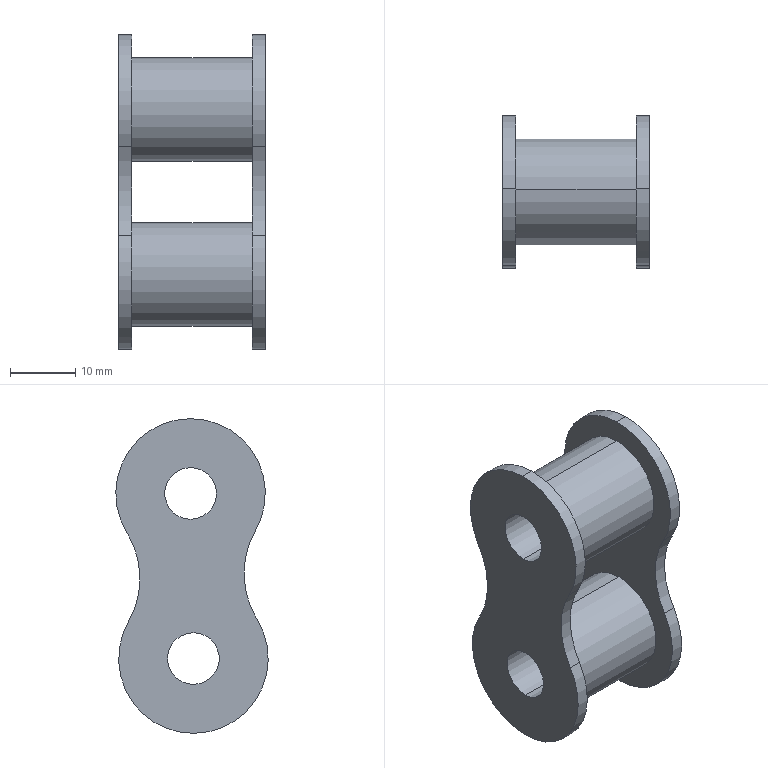Part | STEP file | Mirror 4 | 1 solid | 24 faces | box 22.5 x 23.441 x 48.396 mm | volume 8734 mm3 | cylinder 20 | plane 4 | commonest cylinder face diameters 23 x8 7.94 x4 15.88 x4 26.656 x4
STEP:
#1=CARTESIAN_POINT('',(346.684,-553.033,2506.288));
#2=VERTEX_POINT('',#1);
#3=CARTESIAN_POINT('',(346.684,-563.215,2489.079));
#4=VERTEX_POINT('',#3);
#5=CARTESIAN_POINT('',(346.684,-563.015,2500.578));
#6=DIRECTION('',(-1.,0.,0.));
#7=DIRECTION('',(0.,-0.01735,-0.9998));
#8=AXIS2_PLACEMENT_3D('',#5,#6,#7);
#9=CIRCLE('',#8,11.5);
#10=EDGE_CURVE('',#2,#4,#9,.T.);
#11=ORIENTED_EDGE('',*,*,#10,.T.);
#12=CARTESIAN_POINT('',(344.684,-563.215,2489.079));
#13=VERTEX_POINT('',#12);
#14=CARTESIAN_POINT('',(346.684,-563.215,2489.079));
#15=DIRECTION('',(-1.,0.,0.));
#16=VECTOR('',#15,1000.);
#17=LINE('',#14,#16);
#18=EDGE_CURVE('',#4,#13,#17,.T.);
#19=ORIENTED_EDGE('',*,*,#18,.T.);
#20=CARTESIAN_POINT('',(344.684,-553.033,2506.288));
#21=VERTEX_POINT('',#20);
#22=CARTESIAN_POINT('',(344.684,-563.015,2500.578));
#23=DIRECTION('',(-1.,0.,0.));
#24=DIRECTION('',(0.,-0.01735,-0.9998));
#25=AXIS2_PLACEMENT_3D('',#22,#23,#24);
#26=CIRCLE('',#25,11.5);
#27=EDGE_CURVE('',#21,#13,#26,.T.);
#28=ORIENTED_EDGE('',*,*,#27,.F.);
#29=CARTESIAN_POINT('',(346.684,-553.033,2506.288));
#30=DIRECTION('',(-1.,0.,0.));
#31=VECTOR('',#30,1000.);
#32=LINE('',#29,#31);
#33=EDGE_CURVE('',#2,#21,#32,.T.);
#34=ORIENTED_EDGE('',*,*,#33,.F.);
#35=EDGE_LOOP('',(#11,#19,#28,#34));
#36=FACE_OUTER_BOUND('',#35,.T.);
#37=CARTESIAN_POINT('',(346.684,-563.015,2500.578));
#38=DIRECTION('',(-1.,0.,0.));
#39=DIRECTION('',(0.,-0.01735,-0.9998));
#40=AXIS2_PLACEMENT_3D('',#37,#38,#39);
#41=CYLINDRICAL_SURFACE('',#40,11.5);
#42=ADVANCED_FACE('',(#36),#41,.T.);
#43=CARTESIAN_POINT('',(365.184,-563.215,2489.079));
#44=VERTEX_POINT('',#43);
#45=CARTESIAN_POINT('',(365.184,-572.793,2506.631));
#46=VERTEX_POINT('',#45);
#47=CARTESIAN_POINT('',(365.184,-563.015,2500.578));
#48=DIRECTION('',(-1.,0.,0.));
#49=DIRECTION('',(0.,-0.01735,-0.9998));
#50=AXIS2_PLACEMENT_3D('',#47,#48,#49);
#51=CIRCLE('',#50,11.5);
#52=EDGE_CURVE('',#44,#46,#51,.T.);
#53=ORIENTED_EDGE('',*,*,#52,.F.);
#54=CARTESIAN_POINT('',(367.184,-563.215,2489.079));
#55=VERTEX_POINT('',#54);
#56=CARTESIAN_POINT('',(365.184,-563.215,2489.079));
#57=DIRECTION('',(1.,0.,0.));
#58=VECTOR('',#57,1000.);
#59=LINE('',#56,#58);
#60=EDGE_CURVE('',#44,#55,#59,.T.);
#61=ORIENTED_EDGE('',*,*,#60,.T.);
#62=CARTESIAN_POINT('',(367.184,-572.793,2506.631));
#63=VERTEX_POINT('',#62);
#64=CARTESIAN_POINT('',(367.184,-563.015,2500.578));
#65=DIRECTION('',(-1.,0.,0.));
#66=DIRECTION('',(0.,-0.01735,-0.9998));
#67=AXIS2_PLACEMENT_3D('',#64,#65,#66);
#68=CIRCLE('',#67,11.5);
#69=EDGE_CURVE('',#55,#63,#68,.T.);
#70=ORIENTED_EDGE('',*,*,#69,.T.);
#71=CARTESIAN_POINT('',(365.184,-572.793,2506.631));
#72=DIRECTION('',(1.,0.,0.));
#73=VECTOR('',#72,1000.);
#74=LINE('',#71,#73);
#75=EDGE_CURVE('',#46,#63,#74,.T.);
#76=ORIENTED_EDGE('',*,*,#75,.F.);
#77=EDGE_LOOP('',(#53,#61,#70,#76));
#78=FACE_OUTER_BOUND('',#77,.T.);
#79=CARTESIAN_POINT('',(365.184,-563.015,2500.578));
#80=DIRECTION('',(1.,0.,0.));
#81=DIRECTION('',(0.,-0.01735,-0.9998));
#82=AXIS2_PLACEMENT_3D('',#79,#80,#81);
#83=CYLINDRICAL_SURFACE('',#82,11.5);
#84=ADVANCED_FACE('',(#78),#83,.T.);
#85=CARTESIAN_POINT('',(346.684,-572.557,2520.264));
#86=VERTEX_POINT('',#85);
#87=CARTESIAN_POINT('',(346.684,-562.375,2537.472));
#88=VERTEX_POINT('',#87);
#89=CARTESIAN_POINT('',(346.684,-562.574,2525.974));
#90=DIRECTION('',(-1.,0.,0.));
#91=DIRECTION('',(0.,-0.01735,-0.9998));
#92=AXIS2_PLACEMENT_3D('',#89,#90,#91);
#93=CIRCLE('',#92,11.5);
#94=EDGE_CURVE('',#86,#88,#93,.T.);
#95=ORIENTED_EDGE('',*,*,#94,.T.);
#96=CARTESIAN_POINT('',(344.684,-562.375,2537.472));
#97=VERTEX_POINT('',#96);
#98=CARTESIAN_POINT('',(346.684,-562.375,2537.472));
#99=DIRECTION('',(-1.,0.,0.));
#100=VECTOR('',#99,1000.);
#101=LINE('',#98,#100);
#102=EDGE_CURVE('',#88,#97,#101,.T.);
#103=ORIENTED_EDGE('',*,*,#102,.T.);
#104=CARTESIAN_POINT('',(344.684,-572.557,2520.264));
#105=VERTEX_POINT('',#104);
#106=CARTESIAN_POINT('',(344.684,-562.574,2525.974));
#107=DIRECTION('',(-1.,0.,0.));
#108=DIRECTION('',(0.,-0.01735,-0.9998));
#109=AXIS2_PLACEMENT_3D('',#106,#107,#108);
#110=CIRCLE('',#109,11.5);
#111=EDGE_CURVE('',#105,#97,#110,.T.);
#112=ORIENTED_EDGE('',*,*,#111,.F.);
#113=CARTESIAN_POINT('',(346.684,-572.557,2520.264));
#114=DIRECTION('',(-1.,0.,0.));
#115=VECTOR('',#114,1000.);
#116=LINE('',#113,#115);
#117=EDGE_CURVE('',#86,#105,#116,.T.);
#118=ORIENTED_EDGE('',*,*,#117,.F.);
#119=EDGE_LOOP('',(#95,#103,#112,#118));
#120=FACE_OUTER_BOUND('',#119,.T.);
#121=CARTESIAN_POINT('',(346.684,-562.574,2525.974));
#122=DIRECTION('',(-1.,0.,0.));
#123=DIRECTION('',(0.,-0.01735,-0.9998));
#124=AXIS2_PLACEMENT_3D('',#121,#122,#123);
#125=CYLINDRICAL_SURFACE('',#124,11.5);
#126=ADVANCED_FACE('',(#120),#125,.T.);
#127=CARTESIAN_POINT('',(346.684,-563.153,2492.639));
#128=VERTEX_POINT('',#127);
#129=CARTESIAN_POINT('',(346.684,-562.877,2508.516));
#130=VERTEX_POINT('',#129);
#131=CARTESIAN_POINT('',(346.684,-563.015,2500.578));
#132=DIRECTION('',(-1.,0.,0.));
#133=DIRECTION('',(0.,0.01735,0.9998));
#134=AXIS2_PLACEMENT_3D('',#131,#132,#133);
#135=CIRCLE('',#134,7.94);
#136=EDGE_CURVE('',#128,#130,#135,.T.);
#137=ORIENTED_EDGE('',*,*,#136,.F.);
#138=CARTESIAN_POINT('',(365.184,-563.153,2492.639));
#139=VERTEX_POINT('',#138);
#140=CARTESIAN_POINT('',(355.934,-563.153,2492.639));
#141=DIRECTION('',(-1.,0.,0.));
#142=VECTOR('',#141,1000.);
#143=LINE('',#140,#142);
#144=EDGE_CURVE('',#139,#128,#143,.T.);
#145=ORIENTED_EDGE('',*,*,#144,.F.);
#146=CARTESIAN_POINT('',(365.184,-562.877,2508.516));
#147=VERTEX_POINT('',#146);
#148=CARTESIAN_POINT('',(365.184,-563.015,2500.578));
#149=DIRECTION('',(-1.,0.,0.));
#150=DIRECTION('',(0.,0.01735,0.9998));
#151=AXIS2_PLACEMENT_3D('',#148,#149,#150);
#152=CIRCLE('',#151,7.94);
#153=EDGE_CURVE('',#139,#147,#152,.T.);
#154=ORIENTED_EDGE('',*,*,#153,.T.);
#155=CARTESIAN_POINT('',(355.934,-562.877,2508.516));
#156=DIRECTION('',(-1.,0.,0.));
#157=VECTOR('',#156,1000.);
#158=LINE('',#155,#157);
#159=EDGE_CURVE('',#147,#130,#158,.T.);
#160=ORIENTED_EDGE('',*,*,#159,.T.);
#161=EDGE_LOOP('',(#137,#145,#154,#160));
#162=FACE_OUTER_BOUND('',#161,.T.);
#163=CARTESIAN_POINT('',(355.934,-563.015,2500.578));
#164=DIRECTION('',(1.,0.,0.));
#165=DIRECTION('',(0.,-0.01735,-0.9998));
#166=AXIS2_PLACEMENT_3D('',#163,#164,#165);
#167=CYLINDRICAL_SURFACE('',#166,7.94);
#168=ADVANCED_FACE('',(#162),#167,.T.);
#169=CARTESIAN_POINT('',(346.684,-562.712,2518.035));
#170=VERTEX_POINT('',#169);
#171=CARTESIAN_POINT('',(346.684,-562.437,2533.913));
#172=VERTEX_POINT('',#171);
#173=CARTESIAN_POINT('',(346.684,-562.574,2525.974));
#174=DIRECTION('',(-1.,0.,0.));
#175=DIRECTION('',(0.,-0.01735,-0.9998));
#176=AXIS2_PLACEMENT_3D('',#173,#174,#175);
#177=CIRCLE('',#176,7.94);
#178=EDGE_CURVE('',#170,#172,#177,.T.);
#179=ORIENTED_EDGE('',*,*,#178,.F.);
#180=CARTESIAN_POINT('',(365.184,-562.712,2518.035));
#181=VERTEX_POINT('',#180);
#182=CARTESIAN_POINT('',(355.934,-562.712,2518.035));
#183=DIRECTION('',(-1.,0.,0.));
#184=VECTOR('',#183,1000.);
#185=LINE('',#182,#184);
#186=EDGE_CURVE('',#181,#170,#185,.T.);
#187=ORIENTED_EDGE('',*,*,#186,.F.);
#188=CARTESIAN_POINT('',(365.184,-562.437,2533.913));
#189=VERTEX_POINT('',#188);
#190=CARTESIAN_POINT('',(365.184,-562.574,2525.974));
#191=DIRECTION('',(-1.,0.,0.));
#192=DIRECTION('',(0.,-0.01735,-0.9998));
#193=AXIS2_PLACEMENT_3D('',#190,#191,#192);
#194=CIRCLE('',#193,7.94);
#195=EDGE_CURVE('',#181,#189,#194,.T.);
#196=ORIENTED_EDGE('',*,*,#195,.T.);
#197=CARTESIAN_POINT('',(355.934,-562.437,2533.913));
#198=DIRECTION('',(-1.,0.,0.));
#199=VECTOR('',#198,1000.);
#200=LINE('',#197,#199);
#201=EDGE_CURVE('',#189,#172,#200,.T.);
#202=ORIENTED_EDGE('',*,*,#201,.T.);
#203=EDGE_LOOP('',(#179,#187,#196,#202));
#204=FACE_OUTER_BOUND('',#203,.T.);
#205=CARTESIAN_POINT('',(355.934,-562.574,2525.974));
#206=DIRECTION('',(1.,0.,0.));
#207=DIRECTION('',(0.,-0.01735,-0.9998));
#208=AXIS2_PLACEMENT_3D('',#205,#206,#207);
#209=CYLINDRICAL_SURFACE('',#208,7.94);
#210=ADVANCED_FACE('',(#204),#209,.T.);
#211=CARTESIAN_POINT('',(367.184,-562.506,2529.943));
#212=VERTEX_POINT('',#211);
#213=CARTESIAN_POINT('',(367.184,-562.643,2522.004));
#214=VERTEX_POINT('',#213);
#215=CARTESIAN_POINT('',(367.184,-562.574,2525.974));
#216=DIRECTION('',(-1.,0.,0.));
#217=DIRECTION('',(0.,-0.01735,-0.9998));
#218=AXIS2_PLACEMENT_3D('',#215,#216,#217);
#219=CIRCLE('',#218,3.97);
#220=EDGE_CURVE('',#212,#214,#219,.T.);
#221=ORIENTED_EDGE('',*,*,#220,.F.);
#222=CARTESIAN_POINT('',(344.684,-562.506,2529.943));
#223=VERTEX_POINT('',#222);
#224=CARTESIAN_POINT('',(367.184,-562.506,2529.943));
#225=DIRECTION('',(-1.,0.,0.));
#226=VECTOR('',#225,1000.);
#227=LINE('',#224,#226);
#228=EDGE_CURVE('',#212,#223,#227,.T.);
#229=ORIENTED_EDGE('',*,*,#228,.T.);
#230=CARTESIAN_POINT('',(344.684,-562.643,2522.004));
#231=VERTEX_POINT('',#230);
#232=CARTESIAN_POINT('',(344.684,-562.574,2525.974));
#233=DIRECTION('',(-1.,0.,0.));
#234=DIRECTION('',(0.,-0.01735,-0.9998));
#235=AXIS2_PLACEMENT_3D('',#232,#233,#234);
#236=CIRCLE('',#235,3.97);
#237=EDGE_CURVE('',#223,#231,#236,.T.);
#238=ORIENTED_EDGE('',*,*,#237,.T.);
#239=CARTESIAN_POINT('',(367.184,-562.643,2522.004));
#240=DIRECTION('',(-1.,0.,0.));
#241=VECTOR('',#240,1000.);
#242=LINE('',#239,#241);
#243=EDGE_CURVE('',#214,#231,#242,.T.);
#244=ORIENTED_EDGE('',*,*,#243,.F.);
#245=EDGE_LOOP('',(#221,#229,#238,#244));
#246=FACE_OUTER_BOUND('',#245,.T.);
#247=CARTESIAN_POINT('',(367.184,-562.574,2525.974));
#248=DIRECTION('',(-1.,0.,0.));
#249=DIRECTION('',(0.,0.01735,0.9998));
#250=AXIS2_PLACEMENT_3D('',#247,#248,#249);
#251=CYLINDRICAL_SURFACE('',#250,3.97);
#252=ADVANCED_FACE('',(#246),#251,.F.);
#253=CARTESIAN_POINT('',(367.184,-562.946,2504.547));
#254=VERTEX_POINT('',#253);
#255=CARTESIAN_POINT('',(367.184,-563.084,2496.608));
#256=VERTEX_POINT('',#255);
#257=CARTESIAN_POINT('',(367.184,-563.015,2500.578));
#258=DIRECTION('',(-1.,0.,0.));
#259=DIRECTION('',(0.,0.01735,0.9998));
#260=AXIS2_PLACEMENT_3D('',#257,#258,#259);
#261=CIRCLE('',#260,3.97);
#262=EDGE_CURVE('',#254,#256,#261,.T.);
#263=ORIENTED_EDGE('',*,*,#262,.F.);
#264=CARTESIAN_POINT('',(344.684,-562.946,2504.547));
#265=VERTEX_POINT('',#264);
#266=CARTESIAN_POINT('',(367.184,-562.946,2504.547));
#267=DIRECTION('',(-1.,0.,0.));
#268=VECTOR('',#267,1000.);
#269=LINE('',#266,#268);
#270=EDGE_CURVE('',#254,#265,#269,.T.);
#271=ORIENTED_EDGE('',*,*,#270,.T.);
#272=CARTESIAN_POINT('',(344.684,-563.084,2496.608));
#273=VERTEX_POINT('',#272);
#274=CARTESIAN_POINT('',(344.684,-563.015,2500.578));
#275=DIRECTION('',(-1.,0.,0.));
#276=DIRECTION('',(0.,0.01735,0.9998));
#277=AXIS2_PLACEMENT_3D('',#274,#275,#276);
#278=CIRCLE('',#277,3.97);
#279=EDGE_CURVE('',#265,#273,#278,.T.);
#280=ORIENTED_EDGE('',*,*,#279,.T.);
#281=CARTESIAN_POINT('',(367.184,-563.084,2496.608));
#282=DIRECTION('',(-1.,0.,0.));
#283=VECTOR('',#282,1000.);
#284=LINE('',#281,#283);
#285=EDGE_CURVE('',#256,#273,#284,.T.);
#286=ORIENTED_EDGE('',*,*,#285,.F.);
#287=EDGE_LOOP('',(#263,#271,#280,#286));
#288=FACE_OUTER_BOUND('',#287,.T.);
#289=CARTESIAN_POINT('',(367.184,-563.015,2500.578));
#290=DIRECTION('',(-1.,0.,0.));
#291=DIRECTION('',(0.,0.01735,0.9998));
#292=AXIS2_PLACEMENT_3D('',#289,#290,#291);
#293=CYLINDRICAL_SURFACE('',#292,3.97);
#294=ADVANCED_FACE('',(#288),#293,.F.);
#295=CARTESIAN_POINT('',(365.184,-562.375,2537.472));
#296=VERTEX_POINT('',#295);
#297=CARTESIAN_POINT('',(365.184,-552.796,2519.921));
#298=VERTEX_POINT('',#297);
#299=CARTESIAN_POINT('',(365.184,-562.574,2525.974));
#300=DIRECTION('',(-1.,0.,0.));
#301=DIRECTION('',(0.,-0.01735,-0.9998));
#302=AXIS2_PLACEMENT_3D('',#299,#300,#301);
#303=CIRCLE('',#302,11.5);
#304=EDGE_CURVE('',#296,#298,#303,.T.);
#305=ORIENTED_EDGE('',*,*,#304,.F.);
#306=CARTESIAN_POINT('',(367.184,-562.375,2537.472));
#307=VERTEX_POINT('',#306);
#308=CARTESIAN_POINT('',(365.184,-562.375,2537.472));
#309=DIRECTION('',(1.,0.,0.));
#310=VECTOR('',#309,1000.);
#311=LINE('',#308,#310);
#312=EDGE_CURVE('',#296,#307,#311,.T.);
#313=ORIENTED_EDGE('',*,*,#312,.T.);
#314=CARTESIAN_POINT('',(367.184,-552.796,2519.921));
#315=VERTEX_POINT('',#314);
#316=CARTESIAN_POINT('',(367.184,-562.574,2525.974));
#317=DIRECTION('',(-1.,0.,0.));
#318=DIRECTION('',(0.,-0.01735,-0.9998));
#319=AXIS2_PLACEMENT_3D('',#316,#317,#318);
#320=CIRCLE('',#319,11.5);
#321=EDGE_CURVE('',#307,#315,#320,.T.);
#322=ORIENTED_EDGE('',*,*,#321,.T.);
#323=CARTESIAN_POINT('',(365.184,-552.796,2519.921));
#324=DIRECTION('',(1.,0.,0.));
#325=VECTOR('',#324,1000.);
#326=LINE('',#323,#325);
#327=EDGE_CURVE('',#298,#315,#326,.T.);
#328=ORIENTED_EDGE('',*,*,#327,.F.);
#329=EDGE_LOOP('',(#305,#313,#322,#328));
#330=FACE_OUTER_BOUND('',#329,.T.);
#331=CARTESIAN_POINT('',(365.184,-562.574,2525.974));
#332=DIRECTION('',(1.,0.,0.));
#333=DIRECTION('',(0.,-0.01735,-0.9998));
#334=AXIS2_PLACEMENT_3D('',#331,#332,#333);
#335=CYLINDRICAL_SURFACE('',#334,11.5);
#336=ADVANCED_FACE('',(#330),#335,.T.);
#337=CARTESIAN_POINT('',(365.184,-572.557,2520.264));
#338=VERTEX_POINT('',#337);
#339=CARTESIAN_POINT('',(365.184,-584.126,2513.646));
#340=DIRECTION('',(1.,0.,0.));
#341=DIRECTION('',(0.,0.01735,0.9998));
#342=AXIS2_PLACEMENT_3D('',#339,#340,#341);
#343=CIRCLE('',#342,13.328);
#344=EDGE_CURVE('',#46,#338,#343,.T.);
#345=ORIENTED_EDGE('',*,*,#344,.T.);
#346=CARTESIAN_POINT('',(365.184,-562.574,2525.974));
#347=DIRECTION('',(-1.,0.,0.));
#348=DIRECTION('',(0.,-0.01735,-0.9998));
#349=AXIS2_PLACEMENT_3D('',#346,#347,#348);
#350=CIRCLE('',#349,11.5);
#351=EDGE_CURVE('',#338,#296,#350,.T.);
#352=ORIENTED_EDGE('',*,*,#351,.T.);
#353=ORIENTED_EDGE('',*,*,#304,.T.);
#354=CARTESIAN_POINT('',(365.184,-553.033,2506.288));
#355=VERTEX_POINT('',#354);
#356=CARTESIAN_POINT('',(365.184,-541.464,2512.906));
#357=DIRECTION('',(1.,0.,0.));
#358=DIRECTION('',(0.,-0.01735,-0.9998));
#359=AXIS2_PLACEMENT_3D('',#356,#357,#358);
#360=CIRCLE('',#359,13.328);
#361=EDGE_CURVE('',#298,#355,#360,.T.);
#362=ORIENTED_EDGE('',*,*,#361,.T.);
#363=CARTESIAN_POINT('',(365.184,-563.015,2500.578));
#364=DIRECTION('',(-1.,0.,0.));
#365=DIRECTION('',(0.,-0.01735,-0.9998));
#366=AXIS2_PLACEMENT_3D('',#363,#364,#365);
#367=CIRCLE('',#366,11.5);
#368=EDGE_CURVE('',#355,#44,#367,.T.);
#369=ORIENTED_EDGE('',*,*,#368,.T.);
#370=ORIENTED_EDGE('',*,*,#52,.T.);
#371=EDGE_LOOP('',(#345,#352,#353,#362,#369,#370));
#372=FACE_OUTER_BOUND('',#371,.T.);
#373=CARTESIAN_POINT('',(365.184,-562.574,2525.974));
#374=DIRECTION('',(-1.,0.,0.));
#375=DIRECTION('',(0.,-0.01735,-0.9998));
#376=AXIS2_PLACEMENT_3D('',#373,#374,#375);
#377=CIRCLE('',#376,7.94);
#378=EDGE_CURVE('',#189,#181,#377,.T.);
#379=ORIENTED_EDGE('',*,*,#378,.F.);
#380=ORIENTED_EDGE('',*,*,#195,.F.);
#381=EDGE_LOOP('',(#379,#380));
#382=FACE_BOUND('',#381,.T.);
#383=CARTESIAN_POINT('',(365.184,-563.015,2500.578));
#384=DIRECTION('',(-1.,0.,0.));
#385=DIRECTION('',(0.,0.01735,0.9998));
#386=AXIS2_PLACEMENT_3D('',#383,#384,#385);
#387=CIRCLE('',#386,7.94);
#388=EDGE_CURVE('',#147,#139,#387,.T.);
#389=ORIENTED_EDGE('',*,*,#388,.F.);
#390=ORIENTED_EDGE('',*,*,#153,.F.);
#391=EDGE_LOOP('',(#389,#390));
#392=FACE_BOUND('',#391,.T.);
#393=CARTESIAN_POINT('',(365.184,-573.35,2519.81));
#394=DIRECTION('',(1.,0.,0.));
#395=DIRECTION('',(0.,-0.01735,-0.9998));
#396=AXIS2_PLACEMENT_3D('',#393,#394,#395);
#397=PLANE('',#396);
#398=ADVANCED_FACE('',(#372,#382,#392),#397,.F.);
#399=CARTESIAN_POINT('',(367.184,-572.557,2520.264));
#400=VERTEX_POINT('',#399);
#401=CARTESIAN_POINT('',(367.184,-584.126,2513.646));
#402=DIRECTION('',(1.,0.,0.));
#403=DIRECTION('',(0.,0.01735,0.9998));
#404=AXIS2_PLACEMENT_3D('',#401,#402,#403);
#405=CIRCLE('',#404,13.328);
#406=EDGE_CURVE('',#63,#400,#405,.T.);
#407=ORIENTED_EDGE('',*,*,#406,.T.);
#408=CARTESIAN_POINT('',(365.184,-572.557,2520.264));
#409=DIRECTION('',(1.,0.,0.));
#410=VECTOR('',#409,1000.);
#411=LINE('',#408,#410);
#412=EDGE_CURVE('',#338,#400,#411,.T.);
#413=ORIENTED_EDGE('',*,*,#412,.F.);
#414=ORIENTED_EDGE('',*,*,#344,.F.);
#415=ORIENTED_EDGE('',*,*,#75,.T.);
#416=EDGE_LOOP('',(#407,#413,#414,#415));
#417=FACE_OUTER_BOUND('',#416,.T.);
#418=CARTESIAN_POINT('',(365.184,-584.126,2513.646));
#419=DIRECTION('',(1.,0.,0.));
#420=DIRECTION('',(0.,-0.01735,-0.9998));
#421=AXIS2_PLACEMENT_3D('',#418,#419,#420);
#422=CYLINDRICAL_SURFACE('',#421,13.328);
#423=ADVANCED_FACE('',(#417),#422,.F.);
#424=ORIENTED_EDGE('',*,*,#312,.F.);
#425=ORIENTED_EDGE('',*,*,#351,.F.);
#426=ORIENTED_EDGE('',*,*,#412,.T.);
#427=CARTESIAN_POINT('',(367.184,-562.574,2525.974));
#428=DIRECTION('',(-1.,0.,0.));
#429=DIRECTION('',(0.,-0.01735,-0.9998));
#430=AXIS2_PLACEMENT_3D('',#427,#428,#429);
#431=CIRCLE('',#430,11.5);
#432=EDGE_CURVE('',#400,#307,#431,.T.);
#433=ORIENTED_EDGE('',*,*,#432,.T.);
#434=EDGE_LOOP('',(#424,#425,#426,#433));
#435=FACE_OUTER_BOUND('',#434,.T.);
#436=CARTESIAN_POINT('',(365.184,-562.574,2525.974));
#437=DIRECTION('',(1.,0.,0.));
#438=DIRECTION('',(0.,-0.01735,-0.9998));
#439=AXIS2_PLACEMENT_3D('',#436,#437,#438);
#440=CYLINDRICAL_SURFACE('',#439,11.5);
#441=ADVANCED_FACE('',(#435),#440,.T.);
#442=CARTESIAN_POINT('',(367.184,-553.033,2506.288));
#443=VERTEX_POINT('',#442);
#444=CARTESIAN_POINT('',(367.184,-541.464,2512.906));
#445=DIRECTION('',(1.,0.,0.));
#446=DIRECTION('',(0.,-0.01735,-0.9998));
#447=AXIS2_PLACEMENT_3D('',#444,#445,#446);
#448=CIRCLE('',#447,13.328);
#449=EDGE_CURVE('',#315,#443,#448,.T.);
#450=ORIENTED_EDGE('',*,*,#449,.T.);
#451=CARTESIAN_POINT('',(365.184,-553.033,2506.288));
#452=DIRECTION('',(1.,0.,0.));
#453=VECTOR('',#452,1000.);
#454=LINE('',#451,#453);
#455=EDGE_CURVE('',#355,#443,#454,.T.);
#456=ORIENTED_EDGE('',*,*,#455,.F.);
#457=ORIENTED_EDGE('',*,*,#361,.F.);
#458=ORIENTED_EDGE('',*,*,#327,.T.);
#459=EDGE_LOOP('',(#450,#456,#457,#458));
#460=FACE_OUTER_BOUND('',#459,.T.);
#461=CARTESIAN_POINT('',(365.184,-541.464,2512.906));
#462=DIRECTION('',(1.,0.,0.));
#463=DIRECTION('',(0.,-0.01735,-0.9998));
#464=AXIS2_PLACEMENT_3D('',#461,#462,#463);
#465=CYLINDRICAL_SURFACE('',#464,13.328);
#466=ADVANCED_FACE('',(#460),#465,.F.);
#467=ORIENTED_EDGE('',*,*,#60,.F.);
#468=ORIENTED_EDGE('',*,*,#368,.F.);
#469=ORIENTED_EDGE('',*,*,#455,.T.);
#470=CARTESIAN_POINT('',(367.184,-563.015,2500.578));
#471=DIRECTION('',(-1.,0.,0.));
#472=DIRECTION('',(0.,-0.01735,-0.9998));
#473=AXIS2_PLACEMENT_3D('',#470,#471,#472);
#474=CIRCLE('',#473,11.5);
#475=EDGE_CURVE('',#443,#55,#474,.T.);
#476=ORIENTED_EDGE('',*,*,#475,.T.);
#477=EDGE_LOOP('',(#467,#468,#469,#476));
#478=FACE_OUTER_BOUND('',#477,.T.);
#479=CARTESIAN_POINT('',(365.184,-563.015,2500.578));
#480=DIRECTION('',(1.,0.,0.));
#481=DIRECTION('',(0.,-0.01735,-0.9998));
#482=AXIS2_PLACEMENT_3D('',#479,#480,#481);
#483=CYLINDRICAL_SURFACE('',#482,11.5);
#484=ADVANCED_FACE('',(#478),#483,.T.);
#485=CARTESIAN_POINT('',(367.184,-562.574,2525.974));
#486=DIRECTION('',(-1.,0.,0.));
#487=DIRECTION('',(0.,-0.01735,-0.9998));
#488=AXIS2_PLACEMENT_3D('',#485,#486,#487);
#489=CIRCLE('',#488,3.97);
#490=EDGE_CURVE('',#214,#212,#489,.T.);
#491=ORIENTED_EDGE('',*,*,#490,.T.);
#492=ORIENTED_EDGE('',*,*,#220,.T.);
#493=EDGE_LOOP('',(#491,#492));
#494=FACE_BOUND('',#493,.T.);
#495=CARTESIAN_POINT('',(367.184,-563.015,2500.578));
#496=DIRECTION('',(-1.,0.,0.));
#497=DIRECTION('',(0.,0.01735,0.9998));
#498=AXIS2_PLACEMENT_3D('',#495,#496,#497);
#499=CIRCLE('',#498,3.97);
#500=EDGE_CURVE('',#256,#254,#499,.T.);
#501=ORIENTED_EDGE('',*,*,#500,.T.);
#502=ORIENTED_EDGE('',*,*,#262,.T.);
#503=EDGE_LOOP('',(#501,#502));
#504=FACE_BOUND('',#503,.T.);
#505=ORIENTED_EDGE('',*,*,#406,.F.);
#506=ORIENTED_EDGE('',*,*,#69,.F.);
#507=ORIENTED_EDGE('',*,*,#475,.F.);
#508=ORIENTED_EDGE('',*,*,#449,.F.);
#509=ORIENTED_EDGE('',*,*,#321,.F.);
#510=ORIENTED_EDGE('',*,*,#432,.F.);
#511=EDGE_LOOP('',(#505,#506,#507,#508,#509,#510));
#512=FACE_OUTER_BOUND('',#511,.T.);
#513=CARTESIAN_POINT('',(367.184,-573.35,2519.81));
#514=DIRECTION('',(1.,0.,0.));
#515=DIRECTION('',(0.,-0.01735,-0.9998));
#516=AXIS2_PLACEMENT_3D('',#513,#514,#515);
#517=PLANE('',#516);
#518=ADVANCED_FACE('',(#494,#504,#512),#517,.T.);
#519=ORIENTED_EDGE('',*,*,#270,.F.);
#520=ORIENTED_EDGE('',*,*,#500,.F.);
#521=ORIENTED_EDGE('',*,*,#285,.T.);
#522=CARTESIAN_POINT('',(344.684,-563.015,2500.578));
#523=DIRECTION('',(-1.,0.,0.));
#524=DIRECTION('',(0.,0.01735,0.9998));
#525=AXIS2_PLACEMENT_3D('',#522,#523,#524);
#526=CIRCLE('',#525,3.97);
#527=EDGE_CURVE('',#273,#265,#526,.T.);
#528=ORIENTED_EDGE('',*,*,#527,.T.);
#529=EDGE_LOOP('',(#519,#520,#521,#528));
#530=FACE_OUTER_BOUND('',#529,.T.);
#531=CARTESIAN_POINT('',(367.184,-563.015,2500.578));
#532=DIRECTION('',(-1.,0.,0.));
#533=DIRECTION('',(0.,0.01735,0.9998));
#534=AXIS2_PLACEMENT_3D('',#531,#532,#533);
#535=CYLINDRICAL_SURFACE('',#534,3.97);
#536=ADVANCED_FACE('',(#530),#535,.F.);
#537=ORIENTED_EDGE('',*,*,#228,.F.);
#538=ORIENTED_EDGE('',*,*,#490,.F.);
#539=ORIENTED_EDGE('',*,*,#243,.T.);
#540=CARTESIAN_POINT('',(344.684,-562.574,2525.974));
#541=DIRECTION('',(-1.,0.,0.));
#542=DIRECTION('',(0.,-0.01735,-0.9998));
#543=AXIS2_PLACEMENT_3D('',#540,#541,#542);
#544=CIRCLE('',#543,3.97);
#545=EDGE_CURVE('',#231,#223,#544,.T.);
#546=ORIENTED_EDGE('',*,*,#545,.T.);
#547=EDGE_LOOP('',(#537,#538,#539,#546));
#548=FACE_OUTER_BOUND('',#547,.T.);
#549=CARTESIAN_POINT('',(367.184,-562.574,2525.974));
#550=DIRECTION('',(-1.,0.,0.));
#551=DIRECTION('',(0.,0.01735,0.9998));
#552=AXIS2_PLACEMENT_3D('',#549,#550,#551);
#553=CYLINDRICAL_SURFACE('',#552,3.97);
#554=ADVANCED_FACE('',(#548),#553,.F.);
#555=ORIENTED_EDGE('',*,*,#186,.T.);
#556=CARTESIAN_POINT('',(346.684,-562.574,2525.974));
#557=DIRECTION('',(-1.,0.,0.));
#558=DIRECTION('',(0.,-0.01735,-0.9998));
#559=AXIS2_PLACEMENT_3D('',#556,#557,#558);
#560=CIRCLE('',#559,7.94);
#561=EDGE_CURVE('',#172,#170,#560,.T.);
#562=ORIENTED_EDGE('',*,*,#561,.F.);
#563=ORIENTED_EDGE('',*,*,#201,.F.);
#564=ORIENTED_EDGE('',*,*,#378,.T.);
#565=EDGE_LOOP('',(#555,#562,#563,#564));
#566=FACE_OUTER_BOUND('',#565,.T.);
#567=CARTESIAN_POINT('',(355.934,-562.574,2525.974));
#568=DIRECTION('',(1.,0.,0.));
#569=DIRECTION('',(0.,-0.01735,-0.9998));
#570=AXIS2_PLACEMENT_3D('',#567,#568,#569);
#571=CYLINDRICAL_SURFACE('',#570,7.94);
#572=ADVANCED_FACE('',(#566),#571,.T.);
#573=ORIENTED_EDGE('',*,*,#144,.T.);
#574=CARTESIAN_POINT('',(346.684,-563.015,2500.578));
#575=DIRECTION('',(-1.,0.,0.));
#576=DIRECTION('',(0.,0.01735,0.9998));
#577=AXIS2_PLACEMENT_3D('',#574,#575,#576);
#578=CIRCLE('',#577,7.94);
#579=EDGE_CURVE('',#130,#128,#578,.T.);
#580=ORIENTED_EDGE('',*,*,#579,.F.);
#581=ORIENTED_EDGE('',*,*,#159,.F.);
#582=ORIENTED_EDGE('',*,*,#388,.T.);
#583=EDGE_LOOP('',(#573,#580,#581,#582));
#584=FACE_OUTER_BOUND('',#583,.T.);
#585=CARTESIAN_POINT('',(355.934,-563.015,2500.578));
#586=DIRECTION('',(1.,0.,0.));
#587=DIRECTION('',(0.,-0.01735,-0.9998));
#588=AXIS2_PLACEMENT_3D('',#585,#586,#587);
#589=CYLINDRICAL_SURFACE('',#588,7.94);
#590=ADVANCED_FACE('',(#584),#589,.T.);
#591=CARTESIAN_POINT('',(346.684,-572.793,2506.631));
#592=VERTEX_POINT('',#591);
#593=CARTESIAN_POINT('',(346.684,-584.126,2513.646));
#594=DIRECTION('',(1.,0.,0.));
#595=DIRECTION('',(0.,0.01735,0.9998));
#596=AXIS2_PLACEMENT_3D('',#593,#594,#595);
#597=CIRCLE('',#596,13.328);
#598=EDGE_CURVE('',#592,#86,#597,.T.);
#599=ORIENTED_EDGE('',*,*,#598,.F.);
#600=CARTESIAN_POINT('',(346.684,-563.015,2500.578));
#601=DIRECTION('',(-1.,0.,0.));
#602=DIRECTION('',(0.,-0.01735,-0.9998));
#603=AXIS2_PLACEMENT_3D('',#600,#601,#602);
#604=CIRCLE('',#603,11.5);
#605=EDGE_CURVE('',#4,#592,#604,.T.);
#606=ORIENTED_EDGE('',*,*,#605,.F.);
#607=ORIENTED_EDGE('',*,*,#10,.F.);
#608=CARTESIAN_POINT('',(346.684,-552.796,2519.921));
#609=VERTEX_POINT('',#608);
#610=CARTESIAN_POINT('',(346.684,-541.464,2512.906));
#611=DIRECTION('',(1.,0.,0.));
#612=DIRECTION('',(0.,-0.01735,-0.9998));
#613=AXIS2_PLACEMENT_3D('',#610,#611,#612);
#614=CIRCLE('',#613,13.328);
#615=EDGE_CURVE('',#609,#2,#614,.T.);
#616=ORIENTED_EDGE('',*,*,#615,.F.);
#617=CARTESIAN_POINT('',(346.684,-562.574,2525.974));
#618=DIRECTION('',(-1.,0.,0.));
#619=DIRECTION('',(0.,-0.01735,-0.9998));
#620=AXIS2_PLACEMENT_3D('',#617,#618,#619);
#621=CIRCLE('',#620,11.5);
#622=EDGE_CURVE('',#88,#609,#621,.T.);
#623=ORIENTED_EDGE('',*,*,#622,.F.);
#624=ORIENTED_EDGE('',*,*,#94,.F.);
#625=EDGE_LOOP('',(#599,#606,#607,#616,#623,#624));
#626=FACE_OUTER_BOUND('',#625,.T.);
#627=ORIENTED_EDGE('',*,*,#561,.T.);
#628=ORIENTED_EDGE('',*,*,#178,.T.);
#629=EDGE_LOOP('',(#627,#628));
#630=FACE_BOUND('',#629,.T.);
#631=ORIENTED_EDGE('',*,*,#579,.T.);
#632=ORIENTED_EDGE('',*,*,#136,.T.);
#633=EDGE_LOOP('',(#631,#632));
#634=FACE_BOUND('',#633,.T.);
#635=CARTESIAN_POINT('',(346.684,-573.35,2519.81));
#636=DIRECTION('',(-1.,0.,0.));
#637=DIRECTION('',(0.,-0.01735,-0.9998));
#638=AXIS2_PLACEMENT_3D('',#635,#636,#637);
#639=PLANE('',#638);
#640=ADVANCED_FACE('',(#626,#630,#634),#639,.F.);
#641=CARTESIAN_POINT('',(344.684,-572.793,2506.631));
#642=VERTEX_POINT('',#641);
#643=CARTESIAN_POINT('',(344.684,-584.126,2513.646));
#644=DIRECTION('',(1.,0.,0.));
#645=DIRECTION('',(0.,0.01735,0.9998));
#646=AXIS2_PLACEMENT_3D('',#643,#644,#645);
#647=CIRCLE('',#646,13.328);
#648=EDGE_CURVE('',#642,#105,#647,.T.);
#649=ORIENTED_EDGE('',*,*,#648,.F.);
#650=CARTESIAN_POINT('',(346.684,-572.793,2506.631));
#651=DIRECTION('',(-1.,0.,0.));
#652=VECTOR('',#651,1000.);
#653=LINE('',#650,#652);
#654=EDGE_CURVE('',#592,#642,#653,.T.);
#655=ORIENTED_EDGE('',*,*,#654,.F.);
#656=ORIENTED_EDGE('',*,*,#598,.T.);
#657=ORIENTED_EDGE('',*,*,#117,.T.);
#658=EDGE_LOOP('',(#649,#655,#656,#657));
#659=FACE_OUTER_BOUND('',#658,.T.);
#660=CARTESIAN_POINT('',(346.684,-584.126,2513.646));
#661=DIRECTION('',(-1.,0.,0.));
#662=DIRECTION('',(0.,-0.01735,-0.9998));
#663=AXIS2_PLACEMENT_3D('',#660,#661,#662);
#664=CYLINDRICAL_SURFACE('',#663,13.328);
#665=ADVANCED_FACE('',(#659),#664,.F.);
#666=ORIENTED_EDGE('',*,*,#102,.F.);
#667=ORIENTED_EDGE('',*,*,#622,.T.);
#668=CARTESIAN_POINT('',(344.684,-552.796,2519.921));
#669=VERTEX_POINT('',#668);
#670=CARTESIAN_POINT('',(346.684,-552.796,2519.921));
#671=DIRECTION('',(-1.,0.,0.));
#672=VECTOR('',#671,1000.);
#673=LINE('',#670,#672);
#674=EDGE_CURVE('',#609,#669,#673,.T.);
#675=ORIENTED_EDGE('',*,*,#674,.T.);
#676=CARTESIAN_POINT('',(344.684,-562.574,2525.974));
#677=DIRECTION('',(-1.,0.,0.));
#678=DIRECTION('',(0.,-0.01735,-0.9998));
#679=AXIS2_PLACEMENT_3D('',#676,#677,#678);
#680=CIRCLE('',#679,11.5);
#681=EDGE_CURVE('',#97,#669,#680,.T.);
#682=ORIENTED_EDGE('',*,*,#681,.F.);
#683=EDGE_LOOP('',(#666,#667,#675,#682));
#684=FACE_OUTER_BOUND('',#683,.T.);
#685=CARTESIAN_POINT('',(346.684,-562.574,2525.974));
#686=DIRECTION('',(-1.,0.,0.));
#687=DIRECTION('',(0.,-0.01735,-0.9998));
#688=AXIS2_PLACEMENT_3D('',#685,#686,#687);
#689=CYLINDRICAL_SURFACE('',#688,11.5);
#690=ADVANCED_FACE('',(#684),#689,.T.);
#691=CARTESIAN_POINT('',(344.684,-541.464,2512.906));
#692=DIRECTION('',(1.,0.,0.));
#693=DIRECTION('',(0.,-0.01735,-0.9998));
#694=AXIS2_PLACEMENT_3D('',#691,#692,#693);
#695=CIRCLE('',#694,13.328);
#696=EDGE_CURVE('',#669,#21,#695,.T.);
#697=ORIENTED_EDGE('',*,*,#696,.F.);
#698=ORIENTED_EDGE('',*,*,#674,.F.);
#699=ORIENTED_EDGE('',*,*,#615,.T.);
#700=ORIENTED_EDGE('',*,*,#33,.T.);
#701=EDGE_LOOP('',(#697,#698,#699,#700));
#702=FACE_OUTER_BOUND('',#701,.T.);
#703=CARTESIAN_POINT('',(346.684,-541.464,2512.906));
#704=DIRECTION('',(-1.,0.,0.));
#705=DIRECTION('',(0.,-0.01735,-0.9998));
#706=AXIS2_PLACEMENT_3D('',#703,#704,#705);
#707=CYLINDRICAL_SURFACE('',#706,13.328);
#708=ADVANCED_FACE('',(#702),#707,.F.);
#709=ORIENTED_EDGE('',*,*,#18,.F.);
#710=ORIENTED_EDGE('',*,*,#605,.T.);
#711=ORIENTED_EDGE('',*,*,#654,.T.);
#712=CARTESIAN_POINT('',(344.684,-563.015,2500.578));
#713=DIRECTION('',(-1.,0.,0.));
#714=DIRECTION('',(0.,-0.01735,-0.9998));
#715=AXIS2_PLACEMENT_3D('',#712,#713,#714);
#716=CIRCLE('',#715,11.5);
#717=EDGE_CURVE('',#13,#642,#716,.T.);
#718=ORIENTED_EDGE('',*,*,#717,.F.);
#719=EDGE_LOOP('',(#709,#710,#711,#718));
#720=FACE_OUTER_BOUND('',#719,.T.);
#721=CARTESIAN_POINT('',(346.684,-563.015,2500.578));
#722=DIRECTION('',(-1.,0.,0.));
#723=DIRECTION('',(0.,-0.01735,-0.9998));
#724=AXIS2_PLACEMENT_3D('',#721,#722,#723);
#725=CYLINDRICAL_SURFACE('',#724,11.5);
#726=ADVANCED_FACE('',(#720),#725,.T.);
#727=ORIENTED_EDGE('',*,*,#545,.F.);
#728=ORIENTED_EDGE('',*,*,#237,.F.);
#729=EDGE_LOOP('',(#727,#728));
#730=FACE_BOUND('',#729,.T.);
#731=ORIENTED_EDGE('',*,*,#527,.F.);
#732=ORIENTED_EDGE('',*,*,#279,.F.);
#733=EDGE_LOOP('',(#731,#732));
#734=FACE_BOUND('',#733,.T.);
#735=ORIENTED_EDGE('',*,*,#648,.T.);
#736=ORIENTED_EDGE('',*,*,#111,.T.);
#737=ORIENTED_EDGE('',*,*,#681,.T.);
#738=ORIENTED_EDGE('',*,*,#696,.T.);
#739=ORIENTED_EDGE('',*,*,#27,.T.);
#740=ORIENTED_EDGE('',*,*,#717,.T.);
#741=EDGE_LOOP('',(#735,#736,#737,#738,#739,#740));
#742=FACE_OUTER_BOUND('',#741,.T.);
#743=CARTESIAN_POINT('',(344.684,-573.35,2519.81));
#744=DIRECTION('',(-1.,0.,0.));
#745=DIRECTION('',(0.,-0.01735,-0.9998));
#746=AXIS2_PLACEMENT_3D('',#743,#744,#745);
#747=PLANE('',#746);
#748=ADVANCED_FACE('',(#730,#734,#742),#747,.T.);
#749=CLOSED_SHELL('',(#42,#84,#126,#168,#210,#252,#294,#336,#398,#423,#441,#466,#484,#518,#536,#554,#572,#590,#640,#665,#690,#708,#726,#748));
#750=MANIFOLD_SOLID_BREP('',#749);
#751=CARTESIAN_POINT('',(0.,0.,0.));
#752=DIRECTION('',(0.,0.,1.));
#753=DIRECTION('',(1.,0.,0.));
#754=AXIS2_PLACEMENT_3D('',#751,#752,#753);
#755=(LENGTH_UNIT()NAMED_UNIT(*)SI_UNIT(.MILLI.,.METRE.));
#756=UNCERTAINTY_MEASURE_WITH_UNIT(LENGTH_MEASURE(0.00001),#755,'','');
#757=(NAMED_UNIT(*)PLANE_ANGLE_UNIT()SI_UNIT($,.RADIAN.));
#758=(NAMED_UNIT(*)SI_UNIT($,.STERADIAN.)SOLID_ANGLE_UNIT());
#759=(GEOMETRIC_REPRESENTATION_CONTEXT(3)GLOBAL_UNCERTAINTY_ASSIGNED_CONTEXT((#756))GLOBAL_UNIT_ASSIGNED_CONTEXT((#755,#757,#758))REPRESENTATION_CONTEXT('',''));
#760=ADVANCED_BREP_SHAPE_REPRESENTATION('',(#750,#754),#759);